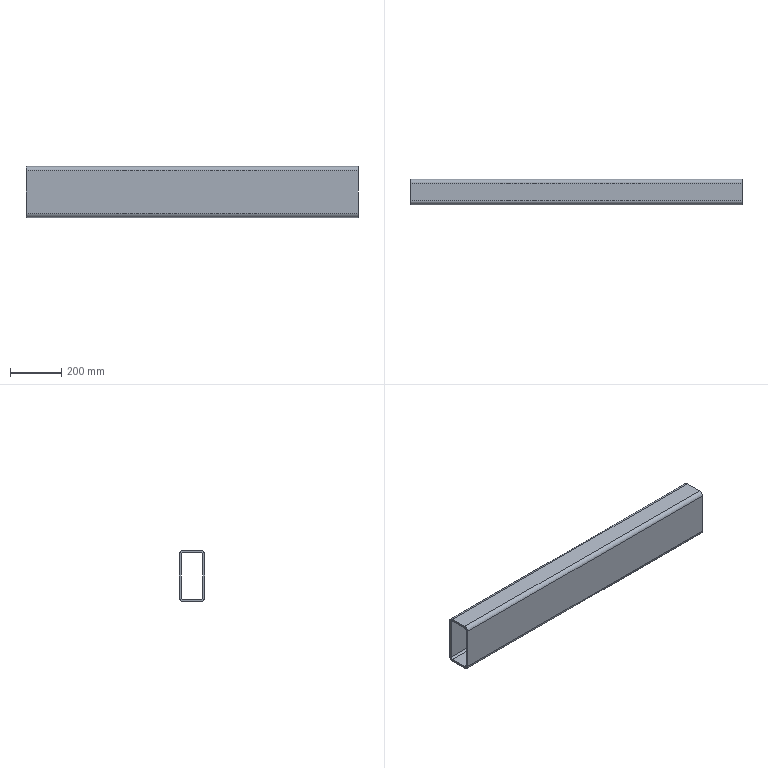Part | STEP file | 01-Column (flat tube 200x100x8)_default<machining> | 1 solid | 18 faces | box 1300 x 100 x 200 mm | volume 5692942 mm3 | plane 10 | cylinder 8 | commonest cylinder face diameters 16 x4 32 x4
STEP:
#1=CARTESIAN_POINT('',(0.,0.,0.));
#2=DIRECTION('',(0.,0.,1.));
#3=DIRECTION('',(1.,0.,0.));
#4=AXIS2_PLACEMENT_3D('',#1,#2,#3);
#5=CARTESIAN_POINT('',(0.,50.,84.));
#6=VERTEX_POINT('',#5);
#7=CARTESIAN_POINT('',(0.,34.,100.));
#8=VERTEX_POINT('',#7);
#9=CARTESIAN_POINT('',(0.,34.,84.));
#10=DIRECTION('',(1.,0.,0.));
#11=DIRECTION('',(0.,0.,-1.));
#12=AXIS2_PLACEMENT_3D('',#9,#10,#11);
#13=CIRCLE('',#12,16.);
#14=CARTESIAN_POINT('',(1300.,34.,84.));
#15=DIRECTION('',(-1.,0.,0.));
#16=DIRECTION('',(0.,0.,1.));
#17=AXIS2_PLACEMENT_3D('',#14,#15,#16);
#18=CYLINDRICAL_SURFACE('',#17,16.);
#19=CARTESIAN_POINT('',(3.142,1300.));
#20=DIRECTION('',(-1.,0.));
#21=VECTOR('',#20,1.);
#22=LINE('',#19,#21);
#23=(GEOMETRIC_REPRESENTATION_CONTEXT(2)PARAMETRIC_REPRESENTATION_CONTEXT()REPRESENTATION_CONTEXT('',''));
#24=DEFINITIONAL_REPRESENTATION('',(#22),#23);
#25=PCURVE('',#18,#24);
#26=CARTESIAN_POINT('',(0.,34.,84.));
#27=DIRECTION('',(1.,0.,0.));
#28=DIRECTION('',(0.,0.,-1.));
#29=AXIS2_PLACEMENT_3D('',#26,#27,#28);
#30=PLANE('',#29);
#31=CARTESIAN_POINT('',(0.,0.));
#32=DIRECTION('',(1.,0.));
#33=AXIS2_PLACEMENT_2D('',#31,#32);
#34=CIRCLE('',#33,16.);
#35=(GEOMETRIC_REPRESENTATION_CONTEXT(2)PARAMETRIC_REPRESENTATION_CONTEXT()REPRESENTATION_CONTEXT('',''));
#36=DEFINITIONAL_REPRESENTATION('',(#34),#35);
#37=PCURVE('',#30,#36);
#38=SURFACE_CURVE('',#13,(#25,#37),.PCURVE_S1.);
#39=EDGE_CURVE('',#6,#8,#38,.T.);
#40=ORIENTED_EDGE('',*,*,#39,.T.);
#41=CARTESIAN_POINT('',(1300.,34.,100.));
#42=VERTEX_POINT('',#41);
#43=CARTESIAN_POINT('',(1300.,34.,100.));
#44=DIRECTION('',(-1.,0.,0.));
#45=VECTOR('',#44,1.);
#46=LINE('',#43,#45);
#47=CARTESIAN_POINT('',(0.,0.));
#48=DIRECTION('',(0.,1.));
#49=VECTOR('',#48,1.);
#50=LINE('',#47,#49);
#51=(GEOMETRIC_REPRESENTATION_CONTEXT(2)PARAMETRIC_REPRESENTATION_CONTEXT()REPRESENTATION_CONTEXT('',''));
#52=DEFINITIONAL_REPRESENTATION('',(#50),#51);
#53=PCURVE('',#18,#52);
#54=CARTESIAN_POINT('',(1300.,34.,100.));
#55=DIRECTION('',(0.,0.,-1.));
#56=DIRECTION('',(-1.,0.,0.));
#57=AXIS2_PLACEMENT_3D('',#54,#55,#56);
#58=PLANE('',#57);
#59=CARTESIAN_POINT('',(0.,0.));
#60=DIRECTION('',(1.,0.));
#61=VECTOR('',#60,1.);
#62=LINE('',#59,#61);
#63=(GEOMETRIC_REPRESENTATION_CONTEXT(2)PARAMETRIC_REPRESENTATION_CONTEXT()REPRESENTATION_CONTEXT('',''));
#64=DEFINITIONAL_REPRESENTATION('',(#62),#63);
#65=PCURVE('',#58,#64);
#66=SURFACE_CURVE('',#46,(#53,#65),.PCURVE_S1.);
#67=EDGE_CURVE('',#42,#8,#66,.T.);
#68=ORIENTED_EDGE('',*,*,#67,.F.);
#69=CARTESIAN_POINT('',(1300.,50.,84.));
#70=VERTEX_POINT('',#69);
#71=CARTESIAN_POINT('',(1300.,34.,84.));
#72=DIRECTION('',(1.,0.,0.));
#73=DIRECTION('',(0.,0.,-1.));
#74=AXIS2_PLACEMENT_3D('',#71,#72,#73);
#75=CIRCLE('',#74,16.);
#76=CARTESIAN_POINT('',(3.142,0.));
#77=DIRECTION('',(-1.,0.));
#78=VECTOR('',#77,1.);
#79=LINE('',#76,#78);
#80=(GEOMETRIC_REPRESENTATION_CONTEXT(2)PARAMETRIC_REPRESENTATION_CONTEXT()REPRESENTATION_CONTEXT('',''));
#81=DEFINITIONAL_REPRESENTATION('',(#79),#80);
#82=PCURVE('',#18,#81);
#83=CARTESIAN_POINT('',(1300.,34.,84.));
#84=DIRECTION('',(1.,0.,0.));
#85=DIRECTION('',(0.,0.,-1.));
#86=AXIS2_PLACEMENT_3D('',#83,#84,#85);
#87=PLANE('',#86);
#88=CARTESIAN_POINT('',(0.,0.));
#89=DIRECTION('',(1.,0.));
#90=AXIS2_PLACEMENT_2D('',#88,#89);
#91=CIRCLE('',#90,16.);
#92=(GEOMETRIC_REPRESENTATION_CONTEXT(2)PARAMETRIC_REPRESENTATION_CONTEXT()REPRESENTATION_CONTEXT('',''));
#93=DEFINITIONAL_REPRESENTATION('',(#91),#92);
#94=PCURVE('',#87,#93);
#95=SURFACE_CURVE('',#75,(#82,#94),.PCURVE_S1.);
#96=EDGE_CURVE('',#70,#42,#95,.T.);
#97=ORIENTED_EDGE('',*,*,#96,.F.);
#98=CARTESIAN_POINT('',(1300.,50.,84.));
#99=DIRECTION('',(-1.,0.,0.));
#100=VECTOR('',#99,1.);
#101=LINE('',#98,#100);
#102=CARTESIAN_POINT('',(1.571,0.));
#103=DIRECTION('',(0.,1.));
#104=VECTOR('',#103,1.);
#105=LINE('',#102,#104);
#106=(GEOMETRIC_REPRESENTATION_CONTEXT(2)PARAMETRIC_REPRESENTATION_CONTEXT()REPRESENTATION_CONTEXT('',''));
#107=DEFINITIONAL_REPRESENTATION('',(#105),#106);
#108=PCURVE('',#18,#107);
#109=CARTESIAN_POINT('',(1300.,50.,84.));
#110=DIRECTION('',(0.,-1.,0.));
#111=DIRECTION('',(0.,0.,-1.));
#112=AXIS2_PLACEMENT_3D('',#109,#110,#111);
#113=PLANE('',#112);
#114=CARTESIAN_POINT('',(0.,0.));
#115=DIRECTION('',(0.,-1.));
#116=VECTOR('',#115,1.);
#117=LINE('',#114,#116);
#118=(GEOMETRIC_REPRESENTATION_CONTEXT(2)PARAMETRIC_REPRESENTATION_CONTEXT()REPRESENTATION_CONTEXT('',''));
#119=DEFINITIONAL_REPRESENTATION('',(#117),#118);
#120=PCURVE('',#113,#119);
#121=SURFACE_CURVE('',#101,(#108,#120),.PCURVE_S1.);
#122=EDGE_CURVE('',#70,#6,#121,.T.);
#123=ORIENTED_EDGE('',*,*,#122,.T.);
#124=EDGE_LOOP('',(#40,#68,#97,#123));
#125=FACE_BOUND('',#124,.T.);
#126=ADVANCED_FACE('',(#125),#18,.T.);
#127=CARTESIAN_POINT('',(0.,-34.,100.));
#128=VERTEX_POINT('',#127);
#129=CARTESIAN_POINT('',(0.,34.,100.));
#130=DIRECTION('',(0.,-1.,0.));
#131=VECTOR('',#130,1.);
#132=LINE('',#129,#131);
#133=CARTESIAN_POINT('',(1300.,0.));
#134=DIRECTION('',(0.,-1.));
#135=VECTOR('',#134,1.);
#136=LINE('',#133,#135);
#137=(GEOMETRIC_REPRESENTATION_CONTEXT(2)PARAMETRIC_REPRESENTATION_CONTEXT()REPRESENTATION_CONTEXT('',''));
#138=DEFINITIONAL_REPRESENTATION('',(#136),#137);
#139=PCURVE('',#58,#138);
#140=CARTESIAN_POINT('',(-16.,0.));
#141=DIRECTION('',(0.,-1.));
#142=VECTOR('',#141,1.);
#143=LINE('',#140,#142);
#144=(GEOMETRIC_REPRESENTATION_CONTEXT(2)PARAMETRIC_REPRESENTATION_CONTEXT()REPRESENTATION_CONTEXT('',''));
#145=DEFINITIONAL_REPRESENTATION('',(#143),#144);
#146=PCURVE('',#30,#145);
#147=SURFACE_CURVE('',#132,(#139,#146),.PCURVE_S1.);
#148=EDGE_CURVE('',#8,#128,#147,.T.);
#149=ORIENTED_EDGE('',*,*,#148,.T.);
#150=CARTESIAN_POINT('',(1300.,-34.,100.));
#151=VERTEX_POINT('',#150);
#152=CARTESIAN_POINT('',(1300.,-34.,100.));
#153=DIRECTION('',(-1.,0.,0.));
#154=VECTOR('',#153,1.);
#155=LINE('',#152,#154);
#156=CARTESIAN_POINT('',(0.,-68.));
#157=DIRECTION('',(1.,0.));
#158=VECTOR('',#157,1.);
#159=LINE('',#156,#158);
#160=(GEOMETRIC_REPRESENTATION_CONTEXT(2)PARAMETRIC_REPRESENTATION_CONTEXT()REPRESENTATION_CONTEXT('',''));
#161=DEFINITIONAL_REPRESENTATION('',(#159),#160);
#162=PCURVE('',#58,#161);
#163=CARTESIAN_POINT('',(1300.,-34.,84.));
#164=DIRECTION('',(-1.,0.,0.));
#165=DIRECTION('',(0.,0.,1.));
#166=AXIS2_PLACEMENT_3D('',#163,#164,#165);
#167=CYLINDRICAL_SURFACE('',#166,16.);
#168=CARTESIAN_POINT('',(6.283,0.));
#169=DIRECTION('',(0.,1.));
#170=VECTOR('',#169,1.);
#171=LINE('',#168,#170);
#172=(GEOMETRIC_REPRESENTATION_CONTEXT(2)PARAMETRIC_REPRESENTATION_CONTEXT()REPRESENTATION_CONTEXT('',''));
#173=DEFINITIONAL_REPRESENTATION('',(#171),#172);
#174=PCURVE('',#167,#173);
#175=SURFACE_CURVE('',#155,(#162,#174),.PCURVE_S1.);
#176=EDGE_CURVE('',#151,#128,#175,.T.);
#177=ORIENTED_EDGE('',*,*,#176,.F.);
#178=CARTESIAN_POINT('',(1300.,34.,100.));
#179=DIRECTION('',(0.,-1.,0.));
#180=VECTOR('',#179,1.);
#181=LINE('',#178,#180);
#182=CARTESIAN_POINT('',(0.,0.));
#183=DIRECTION('',(0.,-1.));
#184=VECTOR('',#183,1.);
#185=LINE('',#182,#184);
#186=(GEOMETRIC_REPRESENTATION_CONTEXT(2)PARAMETRIC_REPRESENTATION_CONTEXT()REPRESENTATION_CONTEXT('',''));
#187=DEFINITIONAL_REPRESENTATION('',(#185),#186);
#188=PCURVE('',#58,#187);
#189=CARTESIAN_POINT('',(-16.,0.));
#190=DIRECTION('',(0.,-1.));
#191=VECTOR('',#190,1.);
#192=LINE('',#189,#191);
#193=(GEOMETRIC_REPRESENTATION_CONTEXT(2)PARAMETRIC_REPRESENTATION_CONTEXT()REPRESENTATION_CONTEXT('',''));
#194=DEFINITIONAL_REPRESENTATION('',(#192),#193);
#195=PCURVE('',#87,#194);
#196=SURFACE_CURVE('',#181,(#188,#195),.PCURVE_S1.);
#197=EDGE_CURVE('',#42,#151,#196,.T.);
#198=ORIENTED_EDGE('',*,*,#197,.F.);
#199=ORIENTED_EDGE('',*,*,#67,.T.);
#200=EDGE_LOOP('',(#149,#177,#198,#199));
#201=FACE_BOUND('',#200,.T.);
#202=ADVANCED_FACE('',(#201),#58,.F.);
#203=CARTESIAN_POINT('',(0.,-50.,84.));
#204=VERTEX_POINT('',#203);
#205=CARTESIAN_POINT('',(0.,-34.,84.));
#206=DIRECTION('',(1.,0.,0.));
#207=DIRECTION('',(0.,0.,-1.));
#208=AXIS2_PLACEMENT_3D('',#205,#206,#207);
#209=CIRCLE('',#208,16.);
#210=CARTESIAN_POINT('',(9.425,1300.));
#211=DIRECTION('',(-1.,0.));
#212=VECTOR('',#211,1.);
#213=LINE('',#210,#212);
#214=(GEOMETRIC_REPRESENTATION_CONTEXT(2)PARAMETRIC_REPRESENTATION_CONTEXT()REPRESENTATION_CONTEXT('',''));
#215=DEFINITIONAL_REPRESENTATION('',(#213),#214);
#216=PCURVE('',#167,#215);
#217=CARTESIAN_POINT('',(0.,-68.));
#218=DIRECTION('',(1.,0.));
#219=AXIS2_PLACEMENT_2D('',#217,#218);
#220=CIRCLE('',#219,16.);
#221=(GEOMETRIC_REPRESENTATION_CONTEXT(2)PARAMETRIC_REPRESENTATION_CONTEXT()REPRESENTATION_CONTEXT('',''));
#222=DEFINITIONAL_REPRESENTATION('',(#220),#221);
#223=PCURVE('',#30,#222);
#224=SURFACE_CURVE('',#209,(#216,#223),.PCURVE_S1.);
#225=EDGE_CURVE('',#128,#204,#224,.T.);
#226=ORIENTED_EDGE('',*,*,#225,.T.);
#227=CARTESIAN_POINT('',(1300.,-50.,84.));
#228=VERTEX_POINT('',#227);
#229=CARTESIAN_POINT('',(1300.,-50.,84.));
#230=DIRECTION('',(-1.,0.,0.));
#231=VECTOR('',#230,1.);
#232=LINE('',#229,#231);
#233=CARTESIAN_POINT('',(4.712,0.));
#234=DIRECTION('',(0.,1.));
#235=VECTOR('',#234,1.);
#236=LINE('',#233,#235);
#237=(GEOMETRIC_REPRESENTATION_CONTEXT(2)PARAMETRIC_REPRESENTATION_CONTEXT()REPRESENTATION_CONTEXT('',''));
#238=DEFINITIONAL_REPRESENTATION('',(#236),#237);
#239=PCURVE('',#167,#238);
#240=CARTESIAN_POINT('',(1300.,-50.,-84.));
#241=DIRECTION('',(0.,1.,0.));
#242=DIRECTION('',(0.,0.,1.));
#243=AXIS2_PLACEMENT_3D('',#240,#241,#242);
#244=PLANE('',#243);
#245=CARTESIAN_POINT('',(168.,0.));
#246=DIRECTION('',(0.,-1.));
#247=VECTOR('',#246,1.);
#248=LINE('',#245,#247);
#249=(GEOMETRIC_REPRESENTATION_CONTEXT(2)PARAMETRIC_REPRESENTATION_CONTEXT()REPRESENTATION_CONTEXT('',''));
#250=DEFINITIONAL_REPRESENTATION('',(#248),#249);
#251=PCURVE('',#244,#250);
#252=SURFACE_CURVE('',#232,(#239,#251),.PCURVE_S1.);
#253=EDGE_CURVE('',#228,#204,#252,.T.);
#254=ORIENTED_EDGE('',*,*,#253,.F.);
#255=CARTESIAN_POINT('',(1300.,-34.,84.));
#256=DIRECTION('',(1.,0.,0.));
#257=DIRECTION('',(0.,0.,-1.));
#258=AXIS2_PLACEMENT_3D('',#255,#256,#257);
#259=CIRCLE('',#258,16.);
#260=CARTESIAN_POINT('',(9.425,0.));
#261=DIRECTION('',(-1.,0.));
#262=VECTOR('',#261,1.);
#263=LINE('',#260,#262);
#264=(GEOMETRIC_REPRESENTATION_CONTEXT(2)PARAMETRIC_REPRESENTATION_CONTEXT()REPRESENTATION_CONTEXT('',''));
#265=DEFINITIONAL_REPRESENTATION('',(#263),#264);
#266=PCURVE('',#167,#265);
#267=CARTESIAN_POINT('',(0.,-68.));
#268=DIRECTION('',(1.,0.));
#269=AXIS2_PLACEMENT_2D('',#267,#268);
#270=CIRCLE('',#269,16.);
#271=(GEOMETRIC_REPRESENTATION_CONTEXT(2)PARAMETRIC_REPRESENTATION_CONTEXT()REPRESENTATION_CONTEXT('',''));
#272=DEFINITIONAL_REPRESENTATION('',(#270),#271);
#273=PCURVE('',#87,#272);
#274=SURFACE_CURVE('',#259,(#266,#273),.PCURVE_S1.);
#275=EDGE_CURVE('',#151,#228,#274,.T.);
#276=ORIENTED_EDGE('',*,*,#275,.F.);
#277=ORIENTED_EDGE('',*,*,#176,.T.);
#278=EDGE_LOOP('',(#226,#254,#276,#277));
#279=FACE_BOUND('',#278,.T.);
#280=ADVANCED_FACE('',(#279),#167,.T.);
#281=CARTESIAN_POINT('',(0.,-50.,-84.));
#282=VERTEX_POINT('',#281);
#283=CARTESIAN_POINT('',(0.,-50.,-84.));
#284=DIRECTION('',(0.,0.,-1.));
#285=VECTOR('',#284,1.);
#286=LINE('',#283,#285);
#287=CARTESIAN_POINT('',(0.,-1300.));
#288=DIRECTION('',(-1.,0.));
#289=VECTOR('',#288,1.);
#290=LINE('',#287,#289);
#291=(GEOMETRIC_REPRESENTATION_CONTEXT(2)PARAMETRIC_REPRESENTATION_CONTEXT()REPRESENTATION_CONTEXT('',''));
#292=DEFINITIONAL_REPRESENTATION('',(#290),#291);
#293=PCURVE('',#244,#292);
#294=CARTESIAN_POINT('',(168.,-84.));
#295=DIRECTION('',(1.,0.));
#296=VECTOR('',#295,1.);
#297=LINE('',#294,#296);
#298=(GEOMETRIC_REPRESENTATION_CONTEXT(2)PARAMETRIC_REPRESENTATION_CONTEXT()REPRESENTATION_CONTEXT('',''));
#299=DEFINITIONAL_REPRESENTATION('',(#297),#298);
#300=PCURVE('',#30,#299);
#301=SURFACE_CURVE('',#286,(#293,#300),.PCURVE_S1.);
#302=EDGE_CURVE('',#204,#282,#301,.T.);
#303=ORIENTED_EDGE('',*,*,#302,.T.);
#304=CARTESIAN_POINT('',(1300.,-50.,-84.));
#305=VERTEX_POINT('',#304);
#306=CARTESIAN_POINT('',(1300.,-50.,-84.));
#307=DIRECTION('',(-1.,0.,0.));
#308=VECTOR('',#307,1.);
#309=LINE('',#306,#308);
#310=CARTESIAN_POINT('',(0.,0.));
#311=DIRECTION('',(0.,-1.));
#312=VECTOR('',#311,1.);
#313=LINE('',#310,#312);
#314=(GEOMETRIC_REPRESENTATION_CONTEXT(2)PARAMETRIC_REPRESENTATION_CONTEXT()REPRESENTATION_CONTEXT('',''));
#315=DEFINITIONAL_REPRESENTATION('',(#313),#314);
#316=PCURVE('',#244,#315);
#317=CARTESIAN_POINT('',(1300.,-34.,-84.));
#318=DIRECTION('',(-1.,0.,0.));
#319=DIRECTION('',(0.,0.,1.));
#320=AXIS2_PLACEMENT_3D('',#317,#318,#319);
#321=CYLINDRICAL_SURFACE('',#320,16.);
#322=CARTESIAN_POINT('',(4.712,0.));
#323=DIRECTION('',(0.,1.));
#324=VECTOR('',#323,1.);
#325=LINE('',#322,#324);
#326=(GEOMETRIC_REPRESENTATION_CONTEXT(2)PARAMETRIC_REPRESENTATION_CONTEXT()REPRESENTATION_CONTEXT('',''));
#327=DEFINITIONAL_REPRESENTATION('',(#325),#326);
#328=PCURVE('',#321,#327);
#329=SURFACE_CURVE('',#309,(#316,#328),.PCURVE_S1.);
#330=EDGE_CURVE('',#305,#282,#329,.T.);
#331=ORIENTED_EDGE('',*,*,#330,.F.);
#332=CARTESIAN_POINT('',(1300.,-50.,-84.));
#333=DIRECTION('',(0.,0.,-1.));
#334=VECTOR('',#333,1.);
#335=LINE('',#332,#334);
#336=CARTESIAN_POINT('',(0.,0.));
#337=DIRECTION('',(-1.,0.));
#338=VECTOR('',#337,1.);
#339=LINE('',#336,#338);
#340=(GEOMETRIC_REPRESENTATION_CONTEXT(2)PARAMETRIC_REPRESENTATION_CONTEXT()REPRESENTATION_CONTEXT('',''));
#341=DEFINITIONAL_REPRESENTATION('',(#339),#340);
#342=PCURVE('',#244,#341);
#343=CARTESIAN_POINT('',(168.,-84.));
#344=DIRECTION('',(1.,0.));
#345=VECTOR('',#344,1.);
#346=LINE('',#343,#345);
#347=(GEOMETRIC_REPRESENTATION_CONTEXT(2)PARAMETRIC_REPRESENTATION_CONTEXT()REPRESENTATION_CONTEXT('',''));
#348=DEFINITIONAL_REPRESENTATION('',(#346),#347);
#349=PCURVE('',#87,#348);
#350=SURFACE_CURVE('',#335,(#342,#349),.PCURVE_S1.);
#351=EDGE_CURVE('',#228,#305,#350,.T.);
#352=ORIENTED_EDGE('',*,*,#351,.F.);
#353=ORIENTED_EDGE('',*,*,#253,.T.);
#354=EDGE_LOOP('',(#303,#331,#352,#353));
#355=FACE_BOUND('',#354,.T.);
#356=ADVANCED_FACE('',(#355),#244,.F.);
#357=CARTESIAN_POINT('',(0.,-34.,-100.));
#358=VERTEX_POINT('',#357);
#359=CARTESIAN_POINT('',(0.,-34.,-84.));
#360=DIRECTION('',(1.,0.,0.));
#361=DIRECTION('',(0.,0.,-1.));
#362=AXIS2_PLACEMENT_3D('',#359,#360,#361);
#363=CIRCLE('',#362,16.);
#364=CARTESIAN_POINT('',(9.425,1300.));
#365=DIRECTION('',(-1.,0.));
#366=VECTOR('',#365,1.);
#367=LINE('',#364,#366);
#368=(GEOMETRIC_REPRESENTATION_CONTEXT(2)PARAMETRIC_REPRESENTATION_CONTEXT()REPRESENTATION_CONTEXT('',''));
#369=DEFINITIONAL_REPRESENTATION('',(#367),#368);
#370=PCURVE('',#321,#369);
#371=CARTESIAN_POINT('',(168.,-68.));
#372=DIRECTION('',(1.,0.));
#373=AXIS2_PLACEMENT_2D('',#371,#372);
#374=CIRCLE('',#373,16.);
#375=(GEOMETRIC_REPRESENTATION_CONTEXT(2)PARAMETRIC_REPRESENTATION_CONTEXT()REPRESENTATION_CONTEXT('',''));
#376=DEFINITIONAL_REPRESENTATION('',(#374),#375);
#377=PCURVE('',#30,#376);
#378=SURFACE_CURVE('',#363,(#370,#377),.PCURVE_S1.);
#379=EDGE_CURVE('',#282,#358,#378,.T.);
#380=ORIENTED_EDGE('',*,*,#379,.T.);
#381=CARTESIAN_POINT('',(1300.,-34.,-100.));
#382=VERTEX_POINT('',#381);
#383=CARTESIAN_POINT('',(1300.,-34.,-100.));
#384=DIRECTION('',(-1.,0.,0.));
#385=VECTOR('',#384,1.);
#386=LINE('',#383,#385);
#387=CARTESIAN_POINT('',(3.142,0.));
#388=DIRECTION('',(0.,1.));
#389=VECTOR('',#388,1.);
#390=LINE('',#387,#389);
#391=(GEOMETRIC_REPRESENTATION_CONTEXT(2)PARAMETRIC_REPRESENTATION_CONTEXT()REPRESENTATION_CONTEXT('',''));
#392=DEFINITIONAL_REPRESENTATION('',(#390),#391);
#393=PCURVE('',#321,#392);
#394=CARTESIAN_POINT('',(1300.,-34.,-100.));
#395=DIRECTION('',(0.,0.,1.));
#396=DIRECTION('',(1.,0.,0.));
#397=AXIS2_PLACEMENT_3D('',#394,#395,#396);
#398=PLANE('',#397);
#399=CARTESIAN_POINT('',(0.,0.));
#400=DIRECTION('',(-1.,0.));
#401=VECTOR('',#400,1.);
#402=LINE('',#399,#401);
#403=(GEOMETRIC_REPRESENTATION_CONTEXT(2)PARAMETRIC_REPRESENTATION_CONTEXT()REPRESENTATION_CONTEXT('',''));
#404=DEFINITIONAL_REPRESENTATION('',(#402),#403);
#405=PCURVE('',#398,#404);
#406=SURFACE_CURVE('',#386,(#393,#405),.PCURVE_S1.);
#407=EDGE_CURVE('',#382,#358,#406,.T.);
#408=ORIENTED_EDGE('',*,*,#407,.F.);
#409=CARTESIAN_POINT('',(1300.,-34.,-84.));
#410=DIRECTION('',(1.,0.,0.));
#411=DIRECTION('',(0.,0.,-1.));
#412=AXIS2_PLACEMENT_3D('',#409,#410,#411);
#413=CIRCLE('',#412,16.);
#414=CARTESIAN_POINT('',(9.425,0.));
#415=DIRECTION('',(-1.,0.));
#416=VECTOR('',#415,1.);
#417=LINE('',#414,#416);
#418=(GEOMETRIC_REPRESENTATION_CONTEXT(2)PARAMETRIC_REPRESENTATION_CONTEXT()REPRESENTATION_CONTEXT('',''));
#419=DEFINITIONAL_REPRESENTATION('',(#417),#418);
#420=PCURVE('',#321,#419);
#421=CARTESIAN_POINT('',(168.,-68.));
#422=DIRECTION('',(1.,0.));
#423=AXIS2_PLACEMENT_2D('',#421,#422);
#424=CIRCLE('',#423,16.);
#425=(GEOMETRIC_REPRESENTATION_CONTEXT(2)PARAMETRIC_REPRESENTATION_CONTEXT()REPRESENTATION_CONTEXT('',''));
#426=DEFINITIONAL_REPRESENTATION('',(#424),#425);
#427=PCURVE('',#87,#426);
#428=SURFACE_CURVE('',#413,(#420,#427),.PCURVE_S1.);
#429=EDGE_CURVE('',#305,#382,#428,.T.);
#430=ORIENTED_EDGE('',*,*,#429,.F.);
#431=ORIENTED_EDGE('',*,*,#330,.T.);
#432=EDGE_LOOP('',(#380,#408,#430,#431));
#433=FACE_BOUND('',#432,.T.);
#434=ADVANCED_FACE('',(#433),#321,.T.);
#435=CARTESIAN_POINT('',(0.,34.,-100.));
#436=VERTEX_POINT('',#435);
#437=CARTESIAN_POINT('',(0.,-34.,-100.));
#438=DIRECTION('',(0.,1.,0.));
#439=VECTOR('',#438,1.);
#440=LINE('',#437,#439);
#441=CARTESIAN_POINT('',(-1300.,0.));
#442=DIRECTION('',(0.,1.));
#443=VECTOR('',#442,1.);
#444=LINE('',#441,#443);
#445=(GEOMETRIC_REPRESENTATION_CONTEXT(2)PARAMETRIC_REPRESENTATION_CONTEXT()REPRESENTATION_CONTEXT('',''));
#446=DEFINITIONAL_REPRESENTATION('',(#444),#445);
#447=PCURVE('',#398,#446);
#448=CARTESIAN_POINT('',(184.,-68.));
#449=DIRECTION('',(0.,1.));
#450=VECTOR('',#449,1.);
#451=LINE('',#448,#450);
#452=(GEOMETRIC_REPRESENTATION_CONTEXT(2)PARAMETRIC_REPRESENTATION_CONTEXT()REPRESENTATION_CONTEXT('',''));
#453=DEFINITIONAL_REPRESENTATION('',(#451),#452);
#454=PCURVE('',#30,#453);
#455=SURFACE_CURVE('',#440,(#447,#454),.PCURVE_S1.);
#456=EDGE_CURVE('',#358,#436,#455,.T.);
#457=ORIENTED_EDGE('',*,*,#456,.T.);
#458=CARTESIAN_POINT('',(1300.,34.,-100.));
#459=VERTEX_POINT('',#458);
#460=CARTESIAN_POINT('',(1300.,34.,-100.));
#461=DIRECTION('',(-1.,0.,0.));
#462=VECTOR('',#461,1.);
#463=LINE('',#460,#462);
#464=CARTESIAN_POINT('',(0.,68.));
#465=DIRECTION('',(-1.,0.));
#466=VECTOR('',#465,1.);
#467=LINE('',#464,#466);
#468=(GEOMETRIC_REPRESENTATION_CONTEXT(2)PARAMETRIC_REPRESENTATION_CONTEXT()REPRESENTATION_CONTEXT('',''));
#469=DEFINITIONAL_REPRESENTATION('',(#467),#468);
#470=PCURVE('',#398,#469);
#471=CARTESIAN_POINT('',(1300.,34.,-84.));
#472=DIRECTION('',(-1.,0.,0.));
#473=DIRECTION('',(0.,0.,1.));
#474=AXIS2_PLACEMENT_3D('',#471,#472,#473);
#475=CYLINDRICAL_SURFACE('',#474,16.);
#476=CARTESIAN_POINT('',(3.142,0.));
#477=DIRECTION('',(0.,1.));
#478=VECTOR('',#477,1.);
#479=LINE('',#476,#478);
#480=(GEOMETRIC_REPRESENTATION_CONTEXT(2)PARAMETRIC_REPRESENTATION_CONTEXT()REPRESENTATION_CONTEXT('',''));
#481=DEFINITIONAL_REPRESENTATION('',(#479),#480);
#482=PCURVE('',#475,#481);
#483=SURFACE_CURVE('',#463,(#470,#482),.PCURVE_S1.);
#484=EDGE_CURVE('',#459,#436,#483,.T.);
#485=ORIENTED_EDGE('',*,*,#484,.F.);
#486=CARTESIAN_POINT('',(1300.,-34.,-100.));
#487=DIRECTION('',(0.,1.,0.));
#488=VECTOR('',#487,1.);
#489=LINE('',#486,#488);
#490=CARTESIAN_POINT('',(0.,0.));
#491=DIRECTION('',(0.,1.));
#492=VECTOR('',#491,1.);
#493=LINE('',#490,#492);
#494=(GEOMETRIC_REPRESENTATION_CONTEXT(2)PARAMETRIC_REPRESENTATION_CONTEXT()REPRESENTATION_CONTEXT('',''));
#495=DEFINITIONAL_REPRESENTATION('',(#493),#494);
#496=PCURVE('',#398,#495);
#497=CARTESIAN_POINT('',(184.,-68.));
#498=DIRECTION('',(0.,1.));
#499=VECTOR('',#498,1.);
#500=LINE('',#497,#499);
#501=(GEOMETRIC_REPRESENTATION_CONTEXT(2)PARAMETRIC_REPRESENTATION_CONTEXT()REPRESENTATION_CONTEXT('',''));
#502=DEFINITIONAL_REPRESENTATION('',(#500),#501);
#503=PCURVE('',#87,#502);
#504=SURFACE_CURVE('',#489,(#496,#503),.PCURVE_S1.);
#505=EDGE_CURVE('',#382,#459,#504,.T.);
#506=ORIENTED_EDGE('',*,*,#505,.F.);
#507=ORIENTED_EDGE('',*,*,#407,.T.);
#508=EDGE_LOOP('',(#457,#485,#506,#507));
#509=FACE_BOUND('',#508,.T.);
#510=ADVANCED_FACE('',(#509),#398,.F.);
#511=CARTESIAN_POINT('',(0.,50.,-84.));
#512=VERTEX_POINT('',#511);
#513=CARTESIAN_POINT('',(0.,34.,-84.));
#514=DIRECTION('',(1.,0.,0.));
#515=DIRECTION('',(0.,0.,-1.));
#516=AXIS2_PLACEMENT_3D('',#513,#514,#515);
#517=CIRCLE('',#516,16.);
#518=CARTESIAN_POINT('',(3.142,1300.));
#519=DIRECTION('',(-1.,0.));
#520=VECTOR('',#519,1.);
#521=LINE('',#518,#520);
#522=(GEOMETRIC_REPRESENTATION_CONTEXT(2)PARAMETRIC_REPRESENTATION_CONTEXT()REPRESENTATION_CONTEXT('',''));
#523=DEFINITIONAL_REPRESENTATION('',(#521),#522);
#524=PCURVE('',#475,#523);
#525=CARTESIAN_POINT('',(168.,0.));
#526=DIRECTION('',(1.,0.));
#527=AXIS2_PLACEMENT_2D('',#525,#526);
#528=CIRCLE('',#527,16.);
#529=(GEOMETRIC_REPRESENTATION_CONTEXT(2)PARAMETRIC_REPRESENTATION_CONTEXT()REPRESENTATION_CONTEXT('',''));
#530=DEFINITIONAL_REPRESENTATION('',(#528),#529);
#531=PCURVE('',#30,#530);
#532=SURFACE_CURVE('',#517,(#524,#531),.PCURVE_S1.);
#533=EDGE_CURVE('',#436,#512,#532,.T.);
#534=ORIENTED_EDGE('',*,*,#533,.T.);
#535=CARTESIAN_POINT('',(1300.,50.,-84.));
#536=VERTEX_POINT('',#535);
#537=CARTESIAN_POINT('',(1300.,50.,-84.));
#538=DIRECTION('',(-1.,0.,0.));
#539=VECTOR('',#538,1.);
#540=LINE('',#537,#539);
#541=CARTESIAN_POINT('',(1.571,0.));
#542=DIRECTION('',(0.,1.));
#543=VECTOR('',#542,1.);
#544=LINE('',#541,#543);
#545=(GEOMETRIC_REPRESENTATION_CONTEXT(2)PARAMETRIC_REPRESENTATION_CONTEXT()REPRESENTATION_CONTEXT('',''));
#546=DEFINITIONAL_REPRESENTATION('',(#544),#545);
#547=PCURVE('',#475,#546);
#548=CARTESIAN_POINT('',(168.,0.));
#549=DIRECTION('',(0.,-1.));
#550=VECTOR('',#549,1.);
#551=LINE('',#548,#550);
#552=(GEOMETRIC_REPRESENTATION_CONTEXT(2)PARAMETRIC_REPRESENTATION_CONTEXT()REPRESENTATION_CONTEXT('',''));
#553=DEFINITIONAL_REPRESENTATION('',(#551),#552);
#554=PCURVE('',#113,#553);
#555=SURFACE_CURVE('',#540,(#547,#554),.PCURVE_S1.);
#556=EDGE_CURVE('',#536,#512,#555,.T.);
#557=ORIENTED_EDGE('',*,*,#556,.F.);
#558=CARTESIAN_POINT('',(1300.,34.,-84.));
#559=DIRECTION('',(1.,0.,0.));
#560=DIRECTION('',(0.,0.,-1.));
#561=AXIS2_PLACEMENT_3D('',#558,#559,#560);
#562=CIRCLE('',#561,16.);
#563=CARTESIAN_POINT('',(3.142,0.));
#564=DIRECTION('',(-1.,0.));
#565=VECTOR('',#564,1.);
#566=LINE('',#563,#565);
#567=(GEOMETRIC_REPRESENTATION_CONTEXT(2)PARAMETRIC_REPRESENTATION_CONTEXT()REPRESENTATION_CONTEXT('',''));
#568=DEFINITIONAL_REPRESENTATION('',(#566),#567);
#569=PCURVE('',#475,#568);
#570=CARTESIAN_POINT('',(168.,0.));
#571=DIRECTION('',(1.,0.));
#572=AXIS2_PLACEMENT_2D('',#570,#571);
#573=CIRCLE('',#572,16.);
#574=(GEOMETRIC_REPRESENTATION_CONTEXT(2)PARAMETRIC_REPRESENTATION_CONTEXT()REPRESENTATION_CONTEXT('',''));
#575=DEFINITIONAL_REPRESENTATION('',(#573),#574);
#576=PCURVE('',#87,#575);
#577=SURFACE_CURVE('',#562,(#569,#576),.PCURVE_S1.);
#578=EDGE_CURVE('',#459,#536,#577,.T.);
#579=ORIENTED_EDGE('',*,*,#578,.F.);
#580=ORIENTED_EDGE('',*,*,#484,.T.);
#581=EDGE_LOOP('',(#534,#557,#579,#580));
#582=FACE_BOUND('',#581,.T.);
#583=ADVANCED_FACE('',(#582),#475,.T.);
#584=CARTESIAN_POINT('',(1300.,-42.,84.));
#585=VERTEX_POINT('',#584);
#586=CARTESIAN_POINT('',(0.,-42.,84.));
#587=VERTEX_POINT('',#586);
#588=CARTESIAN_POINT('',(1300.,-42.,84.));
#589=DIRECTION('',(-1.,0.,0.));
#590=VECTOR('',#589,1.);
#591=LINE('',#588,#590);
#592=CARTESIAN_POINT('',(1300.,-34.,84.));
#593=DIRECTION('',(-1.,0.,0.));
#594=DIRECTION('',(0.,0.,1.));
#595=AXIS2_PLACEMENT_3D('',#592,#593,#594);
#596=CYLINDRICAL_SURFACE('',#595,8.);
#597=CARTESIAN_POINT('',(4.712,0.));
#598=DIRECTION('',(0.,1.));
#599=VECTOR('',#598,1.);
#600=LINE('',#597,#599);
#601=(GEOMETRIC_REPRESENTATION_CONTEXT(2)PARAMETRIC_REPRESENTATION_CONTEXT()REPRESENTATION_CONTEXT('',''));
#602=DEFINITIONAL_REPRESENTATION('',(#600),#601);
#603=PCURVE('',#596,#602);
#604=CARTESIAN_POINT('',(1300.,-42.,-84.));
#605=DIRECTION('',(0.,1.,0.));
#606=DIRECTION('',(0.,0.,1.));
#607=AXIS2_PLACEMENT_3D('',#604,#605,#606);
#608=PLANE('',#607);
#609=CARTESIAN_POINT('',(168.,0.));
#610=DIRECTION('',(0.,-1.));
#611=VECTOR('',#610,1.);
#612=LINE('',#609,#611);
#613=(GEOMETRIC_REPRESENTATION_CONTEXT(2)PARAMETRIC_REPRESENTATION_CONTEXT()REPRESENTATION_CONTEXT('',''));
#614=DEFINITIONAL_REPRESENTATION('',(#612),#613);
#615=PCURVE('',#608,#614);
#616=SURFACE_CURVE('',#591,(#603,#615),.PCURVE_S1.);
#617=EDGE_CURVE('',#585,#587,#616,.T.);
#618=ORIENTED_EDGE('',*,*,#617,.F.);
#619=CARTESIAN_POINT('',(1300.,-34.,92.));
#620=VERTEX_POINT('',#619);
#621=CARTESIAN_POINT('',(1300.,-34.,84.));
#622=DIRECTION('',(1.,0.,0.));
#623=DIRECTION('',(0.,0.,-1.));
#624=AXIS2_PLACEMENT_3D('',#621,#622,#623);
#625=CIRCLE('',#624,8.);
#626=CARTESIAN_POINT('',(9.425,0.));
#627=DIRECTION('',(-1.,0.));
#628=VECTOR('',#627,1.);
#629=LINE('',#626,#628);
#630=(GEOMETRIC_REPRESENTATION_CONTEXT(2)PARAMETRIC_REPRESENTATION_CONTEXT()REPRESENTATION_CONTEXT('',''));
#631=DEFINITIONAL_REPRESENTATION('',(#629),#630);
#632=PCURVE('',#596,#631);
#633=CARTESIAN_POINT('',(0.,-68.));
#634=DIRECTION('',(1.,0.));
#635=AXIS2_PLACEMENT_2D('',#633,#634);
#636=CIRCLE('',#635,8.);
#637=(GEOMETRIC_REPRESENTATION_CONTEXT(2)PARAMETRIC_REPRESENTATION_CONTEXT()REPRESENTATION_CONTEXT('',''));
#638=DEFINITIONAL_REPRESENTATION('',(#636),#637);
#639=PCURVE('',#87,#638);
#640=SURFACE_CURVE('',#625,(#632,#639),.PCURVE_S1.);
#641=EDGE_CURVE('',#620,#585,#640,.T.);
#642=ORIENTED_EDGE('',*,*,#641,.F.);
#643=CARTESIAN_POINT('',(0.,-34.,92.));
#644=VERTEX_POINT('',#643);
#645=CARTESIAN_POINT('',(1300.,-34.,92.));
#646=DIRECTION('',(-1.,0.,0.));
#647=VECTOR('',#646,1.);
#648=LINE('',#645,#647);
#649=CARTESIAN_POINT('',(6.283,0.));
#650=DIRECTION('',(0.,1.));
#651=VECTOR('',#650,1.);
#652=LINE('',#649,#651);
#653=(GEOMETRIC_REPRESENTATION_CONTEXT(2)PARAMETRIC_REPRESENTATION_CONTEXT()REPRESENTATION_CONTEXT('',''));
#654=DEFINITIONAL_REPRESENTATION('',(#652),#653);
#655=PCURVE('',#596,#654);
#656=CARTESIAN_POINT('',(1300.,34.,92.));
#657=DIRECTION('',(0.,0.,-1.));
#658=DIRECTION('',(-1.,0.,0.));
#659=AXIS2_PLACEMENT_3D('',#656,#657,#658);
#660=PLANE('',#659);
#661=CARTESIAN_POINT('',(0.,-68.));
#662=DIRECTION('',(1.,0.));
#663=VECTOR('',#662,1.);
#664=LINE('',#661,#663);
#665=(GEOMETRIC_REPRESENTATION_CONTEXT(2)PARAMETRIC_REPRESENTATION_CONTEXT()REPRESENTATION_CONTEXT('',''));
#666=DEFINITIONAL_REPRESENTATION('',(#664),#665);
#667=PCURVE('',#660,#666);
#668=SURFACE_CURVE('',#648,(#655,#667),.PCURVE_S1.);
#669=EDGE_CURVE('',#620,#644,#668,.T.);
#670=ORIENTED_EDGE('',*,*,#669,.T.);
#671=CARTESIAN_POINT('',(0.,-34.,84.));
#672=DIRECTION('',(1.,0.,0.));
#673=DIRECTION('',(0.,0.,-1.));
#674=AXIS2_PLACEMENT_3D('',#671,#672,#673);
#675=CIRCLE('',#674,8.);
#676=CARTESIAN_POINT('',(9.425,1300.));
#677=DIRECTION('',(-1.,0.));
#678=VECTOR('',#677,1.);
#679=LINE('',#676,#678);
#680=(GEOMETRIC_REPRESENTATION_CONTEXT(2)PARAMETRIC_REPRESENTATION_CONTEXT()REPRESENTATION_CONTEXT('',''));
#681=DEFINITIONAL_REPRESENTATION('',(#679),#680);
#682=PCURVE('',#596,#681);
#683=CARTESIAN_POINT('',(0.,-68.));
#684=DIRECTION('',(1.,0.));
#685=AXIS2_PLACEMENT_2D('',#683,#684);
#686=CIRCLE('',#685,8.);
#687=(GEOMETRIC_REPRESENTATION_CONTEXT(2)PARAMETRIC_REPRESENTATION_CONTEXT()REPRESENTATION_CONTEXT('',''));
#688=DEFINITIONAL_REPRESENTATION('',(#686),#687);
#689=PCURVE('',#30,#688);
#690=SURFACE_CURVE('',#675,(#682,#689),.PCURVE_S1.);
#691=EDGE_CURVE('',#644,#587,#690,.T.);
#692=ORIENTED_EDGE('',*,*,#691,.T.);
#693=EDGE_LOOP('',(#618,#642,#670,#692));
#694=FACE_BOUND('',#693,.F.);
#695=ADVANCED_FACE('',(#694),#596,.F.);
#696=CARTESIAN_POINT('',(0.,34.,92.));
#697=VERTEX_POINT('',#696);
#698=CARTESIAN_POINT('',(0.,34.,92.));
#699=DIRECTION('',(0.,-1.,0.));
#700=VECTOR('',#699,1.);
#701=LINE('',#698,#700);
#702=CARTESIAN_POINT('',(1300.,0.));
#703=DIRECTION('',(0.,-1.));
#704=VECTOR('',#703,1.);
#705=LINE('',#702,#704);
#706=(GEOMETRIC_REPRESENTATION_CONTEXT(2)PARAMETRIC_REPRESENTATION_CONTEXT()REPRESENTATION_CONTEXT('',''));
#707=DEFINITIONAL_REPRESENTATION('',(#705),#706);
#708=PCURVE('',#660,#707);
#709=CARTESIAN_POINT('',(-8.,0.));
#710=DIRECTION('',(0.,-1.));
#711=VECTOR('',#710,1.);
#712=LINE('',#709,#711);
#713=(GEOMETRIC_REPRESENTATION_CONTEXT(2)PARAMETRIC_REPRESENTATION_CONTEXT()REPRESENTATION_CONTEXT('',''));
#714=DEFINITIONAL_REPRESENTATION('',(#712),#713);
#715=PCURVE('',#30,#714);
#716=SURFACE_CURVE('',#701,(#708,#715),.PCURVE_S1.);
#717=EDGE_CURVE('',#697,#644,#716,.T.);
#718=ORIENTED_EDGE('',*,*,#717,.F.);
#719=CARTESIAN_POINT('',(1300.,34.,92.));
#720=VERTEX_POINT('',#719);
#721=CARTESIAN_POINT('',(1300.,34.,92.));
#722=DIRECTION('',(-1.,0.,0.));
#723=VECTOR('',#722,1.);
#724=LINE('',#721,#723);
#725=CARTESIAN_POINT('',(0.,0.));
#726=DIRECTION('',(1.,0.));
#727=VECTOR('',#726,1.);
#728=LINE('',#725,#727);
#729=(GEOMETRIC_REPRESENTATION_CONTEXT(2)PARAMETRIC_REPRESENTATION_CONTEXT()REPRESENTATION_CONTEXT('',''));
#730=DEFINITIONAL_REPRESENTATION('',(#728),#729);
#731=PCURVE('',#660,#730);
#732=CARTESIAN_POINT('',(1300.,34.,84.));
#733=DIRECTION('',(-1.,0.,0.));
#734=DIRECTION('',(0.,0.,1.));
#735=AXIS2_PLACEMENT_3D('',#732,#733,#734);
#736=CYLINDRICAL_SURFACE('',#735,8.);
#737=CARTESIAN_POINT('',(0.,0.));
#738=DIRECTION('',(0.,1.));
#739=VECTOR('',#738,1.);
#740=LINE('',#737,#739);
#741=(GEOMETRIC_REPRESENTATION_CONTEXT(2)PARAMETRIC_REPRESENTATION_CONTEXT()REPRESENTATION_CONTEXT('',''));
#742=DEFINITIONAL_REPRESENTATION('',(#740),#741);
#743=PCURVE('',#736,#742);
#744=SURFACE_CURVE('',#724,(#731,#743),.PCURVE_S1.);
#745=EDGE_CURVE('',#720,#697,#744,.T.);
#746=ORIENTED_EDGE('',*,*,#745,.F.);
#747=CARTESIAN_POINT('',(1300.,34.,92.));
#748=DIRECTION('',(0.,-1.,0.));
#749=VECTOR('',#748,1.);
#750=LINE('',#747,#749);
#751=CARTESIAN_POINT('',(0.,0.));
#752=DIRECTION('',(0.,-1.));
#753=VECTOR('',#752,1.);
#754=LINE('',#751,#753);
#755=(GEOMETRIC_REPRESENTATION_CONTEXT(2)PARAMETRIC_REPRESENTATION_CONTEXT()REPRESENTATION_CONTEXT('',''));
#756=DEFINITIONAL_REPRESENTATION('',(#754),#755);
#757=PCURVE('',#660,#756);
#758=CARTESIAN_POINT('',(-8.,0.));
#759=DIRECTION('',(0.,-1.));
#760=VECTOR('',#759,1.);
#761=LINE('',#758,#760);
#762=(GEOMETRIC_REPRESENTATION_CONTEXT(2)PARAMETRIC_REPRESENTATION_CONTEXT()REPRESENTATION_CONTEXT('',''));
#763=DEFINITIONAL_REPRESENTATION('',(#761),#762);
#764=PCURVE('',#87,#763);
#765=SURFACE_CURVE('',#750,(#757,#764),.PCURVE_S1.);
#766=EDGE_CURVE('',#720,#620,#765,.T.);
#767=ORIENTED_EDGE('',*,*,#766,.T.);
#768=ORIENTED_EDGE('',*,*,#669,.T.);
#769=EDGE_LOOP('',(#718,#746,#767,#768));
#770=FACE_BOUND('',#769,.T.);
#771=ADVANCED_FACE('',(#770),#660,.T.);
#772=ORIENTED_EDGE('',*,*,#745,.F.);
#773=CARTESIAN_POINT('',(1300.,42.,84.));
#774=VERTEX_POINT('',#773);
#775=CARTESIAN_POINT('',(1300.,34.,84.));
#776=DIRECTION('',(1.,0.,0.));
#777=DIRECTION('',(0.,0.,-1.));
#778=AXIS2_PLACEMENT_3D('',#775,#776,#777);
#779=CIRCLE('',#778,8.);
#780=CARTESIAN_POINT('',(3.142,0.));
#781=DIRECTION('',(-1.,0.));
#782=VECTOR('',#781,1.);
#783=LINE('',#780,#782);
#784=(GEOMETRIC_REPRESENTATION_CONTEXT(2)PARAMETRIC_REPRESENTATION_CONTEXT()REPRESENTATION_CONTEXT('',''));
#785=DEFINITIONAL_REPRESENTATION('',(#783),#784);
#786=PCURVE('',#736,#785);
#787=CARTESIAN_POINT('',(0.,0.));
#788=DIRECTION('',(1.,0.));
#789=AXIS2_PLACEMENT_2D('',#787,#788);
#790=CIRCLE('',#789,8.);
#791=(GEOMETRIC_REPRESENTATION_CONTEXT(2)PARAMETRIC_REPRESENTATION_CONTEXT()REPRESENTATION_CONTEXT('',''));
#792=DEFINITIONAL_REPRESENTATION('',(#790),#791);
#793=PCURVE('',#87,#792);
#794=SURFACE_CURVE('',#779,(#786,#793),.PCURVE_S1.);
#795=EDGE_CURVE('',#774,#720,#794,.T.);
#796=ORIENTED_EDGE('',*,*,#795,.F.);
#797=CARTESIAN_POINT('',(0.,42.,84.));
#798=VERTEX_POINT('',#797);
#799=CARTESIAN_POINT('',(1300.,42.,84.));
#800=DIRECTION('',(-1.,0.,0.));
#801=VECTOR('',#800,1.);
#802=LINE('',#799,#801);
#803=CARTESIAN_POINT('',(1.571,0.));
#804=DIRECTION('',(0.,1.));
#805=VECTOR('',#804,1.);
#806=LINE('',#803,#805);
#807=(GEOMETRIC_REPRESENTATION_CONTEXT(2)PARAMETRIC_REPRESENTATION_CONTEXT()REPRESENTATION_CONTEXT('',''));
#808=DEFINITIONAL_REPRESENTATION('',(#806),#807);
#809=PCURVE('',#736,#808);
#810=CARTESIAN_POINT('',(1300.,42.,84.));
#811=DIRECTION('',(0.,-1.,0.));
#812=DIRECTION('',(0.,0.,-1.));
#813=AXIS2_PLACEMENT_3D('',#810,#811,#812);
#814=PLANE('',#813);
#815=CARTESIAN_POINT('',(0.,0.));
#816=DIRECTION('',(0.,-1.));
#817=VECTOR('',#816,1.);
#818=LINE('',#815,#817);
#819=(GEOMETRIC_REPRESENTATION_CONTEXT(2)PARAMETRIC_REPRESENTATION_CONTEXT()REPRESENTATION_CONTEXT('',''));
#820=DEFINITIONAL_REPRESENTATION('',(#818),#819);
#821=PCURVE('',#814,#820);
#822=SURFACE_CURVE('',#802,(#809,#821),.PCURVE_S1.);
#823=EDGE_CURVE('',#774,#798,#822,.T.);
#824=ORIENTED_EDGE('',*,*,#823,.T.);
#825=CARTESIAN_POINT('',(0.,34.,84.));
#826=DIRECTION('',(1.,0.,0.));
#827=DIRECTION('',(0.,0.,-1.));
#828=AXIS2_PLACEMENT_3D('',#825,#826,#827);
#829=CIRCLE('',#828,8.);
#830=CARTESIAN_POINT('',(3.142,1300.));
#831=DIRECTION('',(-1.,0.));
#832=VECTOR('',#831,1.);
#833=LINE('',#830,#832);
#834=(GEOMETRIC_REPRESENTATION_CONTEXT(2)PARAMETRIC_REPRESENTATION_CONTEXT()REPRESENTATION_CONTEXT('',''));
#835=DEFINITIONAL_REPRESENTATION('',(#833),#834);
#836=PCURVE('',#736,#835);
#837=CARTESIAN_POINT('',(0.,0.));
#838=DIRECTION('',(1.,0.));
#839=AXIS2_PLACEMENT_2D('',#837,#838);
#840=CIRCLE('',#839,8.);
#841=(GEOMETRIC_REPRESENTATION_CONTEXT(2)PARAMETRIC_REPRESENTATION_CONTEXT()REPRESENTATION_CONTEXT('',''));
#842=DEFINITIONAL_REPRESENTATION('',(#840),#841);
#843=PCURVE('',#30,#842);
#844=SURFACE_CURVE('',#829,(#836,#843),.PCURVE_S1.);
#845=EDGE_CURVE('',#798,#697,#844,.T.);
#846=ORIENTED_EDGE('',*,*,#845,.T.);
#847=EDGE_LOOP('',(#772,#796,#824,#846));
#848=FACE_BOUND('',#847,.F.);
#849=ADVANCED_FACE('',(#848),#736,.F.);
#850=CARTESIAN_POINT('',(0.,42.,-84.));
#851=VERTEX_POINT('',#850);
#852=CARTESIAN_POINT('',(0.,42.,84.));
#853=DIRECTION('',(0.,0.,1.));
#854=VECTOR('',#853,1.);
#855=LINE('',#852,#854);
#856=CARTESIAN_POINT('',(0.,-1300.));
#857=DIRECTION('',(-1.,0.));
#858=VECTOR('',#857,1.);
#859=LINE('',#856,#858);
#860=(GEOMETRIC_REPRESENTATION_CONTEXT(2)PARAMETRIC_REPRESENTATION_CONTEXT()REPRESENTATION_CONTEXT('',''));
#861=DEFINITIONAL_REPRESENTATION('',(#859),#860);
#862=PCURVE('',#814,#861);
#863=CARTESIAN_POINT('',(0.,8.));
#864=DIRECTION('',(-1.,0.));
#865=VECTOR('',#864,1.);
#866=LINE('',#863,#865);
#867=(GEOMETRIC_REPRESENTATION_CONTEXT(2)PARAMETRIC_REPRESENTATION_CONTEXT()REPRESENTATION_CONTEXT('',''));
#868=DEFINITIONAL_REPRESENTATION('',(#866),#867);
#869=PCURVE('',#30,#868);
#870=SURFACE_CURVE('',#855,(#862,#869),.PCURVE_S1.);
#871=EDGE_CURVE('',#851,#798,#870,.T.);
#872=ORIENTED_EDGE('',*,*,#871,.F.);
#873=CARTESIAN_POINT('',(1300.,42.,-84.));
#874=VERTEX_POINT('',#873);
#875=CARTESIAN_POINT('',(1300.,42.,-84.));
#876=DIRECTION('',(-1.,0.,0.));
#877=VECTOR('',#876,1.);
#878=LINE('',#875,#877);
#879=CARTESIAN_POINT('',(168.,0.));
#880=DIRECTION('',(0.,-1.));
#881=VECTOR('',#880,1.);
#882=LINE('',#879,#881);
#883=(GEOMETRIC_REPRESENTATION_CONTEXT(2)PARAMETRIC_REPRESENTATION_CONTEXT()REPRESENTATION_CONTEXT('',''));
#884=DEFINITIONAL_REPRESENTATION('',(#882),#883);
#885=PCURVE('',#814,#884);
#886=CARTESIAN_POINT('',(1300.,34.,-84.));
#887=DIRECTION('',(-1.,0.,0.));
#888=DIRECTION('',(0.,0.,1.));
#889=AXIS2_PLACEMENT_3D('',#886,#887,#888);
#890=CYLINDRICAL_SURFACE('',#889,8.);
#891=CARTESIAN_POINT('',(1.571,0.));
#892=DIRECTION('',(0.,1.));
#893=VECTOR('',#892,1.);
#894=LINE('',#891,#893);
#895=(GEOMETRIC_REPRESENTATION_CONTEXT(2)PARAMETRIC_REPRESENTATION_CONTEXT()REPRESENTATION_CONTEXT('',''));
#896=DEFINITIONAL_REPRESENTATION('',(#894),#895);
#897=PCURVE('',#890,#896);
#898=SURFACE_CURVE('',#878,(#885,#897),.PCURVE_S1.);
#899=EDGE_CURVE('',#874,#851,#898,.T.);
#900=ORIENTED_EDGE('',*,*,#899,.F.);
#901=CARTESIAN_POINT('',(1300.,42.,84.));
#902=DIRECTION('',(0.,0.,1.));
#903=VECTOR('',#902,1.);
#904=LINE('',#901,#903);
#905=CARTESIAN_POINT('',(0.,0.));
#906=DIRECTION('',(-1.,0.));
#907=VECTOR('',#906,1.);
#908=LINE('',#905,#907);
#909=(GEOMETRIC_REPRESENTATION_CONTEXT(2)PARAMETRIC_REPRESENTATION_CONTEXT()REPRESENTATION_CONTEXT('',''));
#910=DEFINITIONAL_REPRESENTATION('',(#908),#909);
#911=PCURVE('',#814,#910);
#912=CARTESIAN_POINT('',(0.,8.));
#913=DIRECTION('',(-1.,0.));
#914=VECTOR('',#913,1.);
#915=LINE('',#912,#914);
#916=(GEOMETRIC_REPRESENTATION_CONTEXT(2)PARAMETRIC_REPRESENTATION_CONTEXT()REPRESENTATION_CONTEXT('',''));
#917=DEFINITIONAL_REPRESENTATION('',(#915),#916);
#918=PCURVE('',#87,#917);
#919=SURFACE_CURVE('',#904,(#911,#918),.PCURVE_S1.);
#920=EDGE_CURVE('',#874,#774,#919,.T.);
#921=ORIENTED_EDGE('',*,*,#920,.T.);
#922=ORIENTED_EDGE('',*,*,#823,.T.);
#923=EDGE_LOOP('',(#872,#900,#921,#922));
#924=FACE_BOUND('',#923,.T.);
#925=ADVANCED_FACE('',(#924),#814,.T.);
#926=ORIENTED_EDGE('',*,*,#899,.F.);
#927=CARTESIAN_POINT('',(1300.,34.,-92.));
#928=VERTEX_POINT('',#927);
#929=CARTESIAN_POINT('',(1300.,34.,-84.));
#930=DIRECTION('',(1.,0.,0.));
#931=DIRECTION('',(0.,0.,-1.));
#932=AXIS2_PLACEMENT_3D('',#929,#930,#931);
#933=CIRCLE('',#932,8.);
#934=CARTESIAN_POINT('',(3.142,0.));
#935=DIRECTION('',(-1.,0.));
#936=VECTOR('',#935,1.);
#937=LINE('',#934,#936);
#938=(GEOMETRIC_REPRESENTATION_CONTEXT(2)PARAMETRIC_REPRESENTATION_CONTEXT()REPRESENTATION_CONTEXT('',''));
#939=DEFINITIONAL_REPRESENTATION('',(#937),#938);
#940=PCURVE('',#890,#939);
#941=CARTESIAN_POINT('',(168.,0.));
#942=DIRECTION('',(1.,0.));
#943=AXIS2_PLACEMENT_2D('',#941,#942);
#944=CIRCLE('',#943,8.);
#945=(GEOMETRIC_REPRESENTATION_CONTEXT(2)PARAMETRIC_REPRESENTATION_CONTEXT()REPRESENTATION_CONTEXT('',''));
#946=DEFINITIONAL_REPRESENTATION('',(#944),#945);
#947=PCURVE('',#87,#946);
#948=SURFACE_CURVE('',#933,(#940,#947),.PCURVE_S1.);
#949=EDGE_CURVE('',#928,#874,#948,.T.);
#950=ORIENTED_EDGE('',*,*,#949,.F.);
#951=CARTESIAN_POINT('',(0.,34.,-92.));
#952=VERTEX_POINT('',#951);
#953=CARTESIAN_POINT('',(1300.,34.,-92.));
#954=DIRECTION('',(-1.,0.,0.));
#955=VECTOR('',#954,1.);
#956=LINE('',#953,#955);
#957=CARTESIAN_POINT('',(3.142,0.));
#958=DIRECTION('',(0.,1.));
#959=VECTOR('',#958,1.);
#960=LINE('',#957,#959);
#961=(GEOMETRIC_REPRESENTATION_CONTEXT(2)PARAMETRIC_REPRESENTATION_CONTEXT()REPRESENTATION_CONTEXT('',''));
#962=DEFINITIONAL_REPRESENTATION('',(#960),#961);
#963=PCURVE('',#890,#962);
#964=CARTESIAN_POINT('',(1300.,-34.,-92.));
#965=DIRECTION('',(0.,0.,1.));
#966=DIRECTION('',(1.,0.,0.));
#967=AXIS2_PLACEMENT_3D('',#964,#965,#966);
#968=PLANE('',#967);
#969=CARTESIAN_POINT('',(0.,68.));
#970=DIRECTION('',(-1.,0.));
#971=VECTOR('',#970,1.);
#972=LINE('',#969,#971);
#973=(GEOMETRIC_REPRESENTATION_CONTEXT(2)PARAMETRIC_REPRESENTATION_CONTEXT()REPRESENTATION_CONTEXT('',''));
#974=DEFINITIONAL_REPRESENTATION('',(#972),#973);
#975=PCURVE('',#968,#974);
#976=SURFACE_CURVE('',#956,(#963,#975),.PCURVE_S1.);
#977=EDGE_CURVE('',#928,#952,#976,.T.);
#978=ORIENTED_EDGE('',*,*,#977,.T.);
#979=CARTESIAN_POINT('',(0.,34.,-84.));
#980=DIRECTION('',(1.,0.,0.));
#981=DIRECTION('',(0.,0.,-1.));
#982=AXIS2_PLACEMENT_3D('',#979,#980,#981);
#983=CIRCLE('',#982,8.);
#984=CARTESIAN_POINT('',(3.142,1300.));
#985=DIRECTION('',(-1.,0.));
#986=VECTOR('',#985,1.);
#987=LINE('',#984,#986);
#988=(GEOMETRIC_REPRESENTATION_CONTEXT(2)PARAMETRIC_REPRESENTATION_CONTEXT()REPRESENTATION_CONTEXT('',''));
#989=DEFINITIONAL_REPRESENTATION('',(#987),#988);
#990=PCURVE('',#890,#989);
#991=CARTESIAN_POINT('',(168.,0.));
#992=DIRECTION('',(1.,0.));
#993=AXIS2_PLACEMENT_2D('',#991,#992);
#994=CIRCLE('',#993,8.);
#995=(GEOMETRIC_REPRESENTATION_CONTEXT(2)PARAMETRIC_REPRESENTATION_CONTEXT()REPRESENTATION_CONTEXT('',''));
#996=DEFINITIONAL_REPRESENTATION('',(#994),#995);
#997=PCURVE('',#30,#996);
#998=SURFACE_CURVE('',#983,(#990,#997),.PCURVE_S1.);
#999=EDGE_CURVE('',#952,#851,#998,.T.);
#1000=ORIENTED_EDGE('',*,*,#999,.T.);
#1001=EDGE_LOOP('',(#926,#950,#978,#1000));
#1002=FACE_BOUND('',#1001,.F.);
#1003=ADVANCED_FACE('',(#1002),#890,.F.);
#1004=CARTESIAN_POINT('',(0.,-34.,-92.));
#1005=VERTEX_POINT('',#1004);
#1006=CARTESIAN_POINT('',(0.,-34.,-92.));
#1007=DIRECTION('',(0.,1.,0.));
#1008=VECTOR('',#1007,1.);
#1009=LINE('',#1006,#1008);
#1010=CARTESIAN_POINT('',(-1300.,0.));
#1011=DIRECTION('',(0.,1.));
#1012=VECTOR('',#1011,1.);
#1013=LINE('',#1010,#1012);
#1014=(GEOMETRIC_REPRESENTATION_CONTEXT(2)PARAMETRIC_REPRESENTATION_CONTEXT()REPRESENTATION_CONTEXT('',''));
#1015=DEFINITIONAL_REPRESENTATION('',(#1013),#1014);
#1016=PCURVE('',#968,#1015);
#1017=CARTESIAN_POINT('',(176.,-68.));
#1018=DIRECTION('',(0.,1.));
#1019=VECTOR('',#1018,1.);
#1020=LINE('',#1017,#1019);
#1021=(GEOMETRIC_REPRESENTATION_CONTEXT(2)PARAMETRIC_REPRESENTATION_CONTEXT()REPRESENTATION_CONTEXT('',''));
#1022=DEFINITIONAL_REPRESENTATION('',(#1020),#1021);
#1023=PCURVE('',#30,#1022);
#1024=SURFACE_CURVE('',#1009,(#1016,#1023),.PCURVE_S1.);
#1025=EDGE_CURVE('',#1005,#952,#1024,.T.);
#1026=ORIENTED_EDGE('',*,*,#1025,.F.);
#1027=CARTESIAN_POINT('',(1300.,-34.,-92.));
#1028=VERTEX_POINT('',#1027);
#1029=CARTESIAN_POINT('',(1300.,-34.,-92.));
#1030=DIRECTION('',(-1.,0.,0.));
#1031=VECTOR('',#1030,1.);
#1032=LINE('',#1029,#1031);
#1033=CARTESIAN_POINT('',(0.,0.));
#1034=DIRECTION('',(-1.,0.));
#1035=VECTOR('',#1034,1.);
#1036=LINE('',#1033,#1035);
#1037=(GEOMETRIC_REPRESENTATION_CONTEXT(2)PARAMETRIC_REPRESENTATION_CONTEXT()REPRESENTATION_CONTEXT('',''));
#1038=DEFINITIONAL_REPRESENTATION('',(#1036),#1037);
#1039=PCURVE('',#968,#1038);
#1040=CARTESIAN_POINT('',(1300.,-34.,-84.));
#1041=DIRECTION('',(-1.,0.,0.));
#1042=DIRECTION('',(0.,0.,1.));
#1043=AXIS2_PLACEMENT_3D('',#1040,#1041,#1042);
#1044=CYLINDRICAL_SURFACE('',#1043,8.);
#1045=CARTESIAN_POINT('',(3.142,0.));
#1046=DIRECTION('',(0.,1.));
#1047=VECTOR('',#1046,1.);
#1048=LINE('',#1045,#1047);
#1049=(GEOMETRIC_REPRESENTATION_CONTEXT(2)PARAMETRIC_REPRESENTATION_CONTEXT()REPRESENTATION_CONTEXT('',''));
#1050=DEFINITIONAL_REPRESENTATION('',(#1048),#1049);
#1051=PCURVE('',#1044,#1050);
#1052=SURFACE_CURVE('',#1032,(#1039,#1051),.PCURVE_S1.);
#1053=EDGE_CURVE('',#1028,#1005,#1052,.T.);
#1054=ORIENTED_EDGE('',*,*,#1053,.F.);
#1055=CARTESIAN_POINT('',(1300.,-34.,-92.));
#1056=DIRECTION('',(0.,1.,0.));
#1057=VECTOR('',#1056,1.);
#1058=LINE('',#1055,#1057);
#1059=CARTESIAN_POINT('',(0.,0.));
#1060=DIRECTION('',(0.,1.));
#1061=VECTOR('',#1060,1.);
#1062=LINE('',#1059,#1061);
#1063=(GEOMETRIC_REPRESENTATION_CONTEXT(2)PARAMETRIC_REPRESENTATION_CONTEXT()REPRESENTATION_CONTEXT('',''));
#1064=DEFINITIONAL_REPRESENTATION('',(#1062),#1063);
#1065=PCURVE('',#968,#1064);
#1066=CARTESIAN_POINT('',(176.,-68.));
#1067=DIRECTION('',(0.,1.));
#1068=VECTOR('',#1067,1.);
#1069=LINE('',#1066,#1068);
#1070=(GEOMETRIC_REPRESENTATION_CONTEXT(2)PARAMETRIC_REPRESENTATION_CONTEXT()REPRESENTATION_CONTEXT('',''));
#1071=DEFINITIONAL_REPRESENTATION('',(#1069),#1070);
#1072=PCURVE('',#87,#1071);
#1073=SURFACE_CURVE('',#1058,(#1065,#1072),.PCURVE_S1.);
#1074=EDGE_CURVE('',#1028,#928,#1073,.T.);
#1075=ORIENTED_EDGE('',*,*,#1074,.T.);
#1076=ORIENTED_EDGE('',*,*,#977,.T.);
#1077=EDGE_LOOP('',(#1026,#1054,#1075,#1076));
#1078=FACE_BOUND('',#1077,.T.);
#1079=ADVANCED_FACE('',(#1078),#968,.T.);
#1080=ORIENTED_EDGE('',*,*,#1053,.F.);
#1081=CARTESIAN_POINT('',(1300.,-42.,-84.));
#1082=VERTEX_POINT('',#1081);
#1083=CARTESIAN_POINT('',(1300.,-34.,-84.));
#1084=DIRECTION('',(1.,0.,0.));
#1085=DIRECTION('',(0.,0.,-1.));
#1086=AXIS2_PLACEMENT_3D('',#1083,#1084,#1085);
#1087=CIRCLE('',#1086,8.);
#1088=CARTESIAN_POINT('',(9.425,0.));
#1089=DIRECTION('',(-1.,0.));
#1090=VECTOR('',#1089,1.);
#1091=LINE('',#1088,#1090);
#1092=(GEOMETRIC_REPRESENTATION_CONTEXT(2)PARAMETRIC_REPRESENTATION_CONTEXT()REPRESENTATION_CONTEXT('',''));
#1093=DEFINITIONAL_REPRESENTATION('',(#1091),#1092);
#1094=PCURVE('',#1044,#1093);
#1095=CARTESIAN_POINT('',(168.,-68.));
#1096=DIRECTION('',(1.,0.));
#1097=AXIS2_PLACEMENT_2D('',#1095,#1096);
#1098=CIRCLE('',#1097,8.);
#1099=(GEOMETRIC_REPRESENTATION_CONTEXT(2)PARAMETRIC_REPRESENTATION_CONTEXT()REPRESENTATION_CONTEXT('',''));
#1100=DEFINITIONAL_REPRESENTATION('',(#1098),#1099);
#1101=PCURVE('',#87,#1100);
#1102=SURFACE_CURVE('',#1087,(#1094,#1101),.PCURVE_S1.);
#1103=EDGE_CURVE('',#1082,#1028,#1102,.T.);
#1104=ORIENTED_EDGE('',*,*,#1103,.F.);
#1105=CARTESIAN_POINT('',(0.,-42.,-84.));
#1106=VERTEX_POINT('',#1105);
#1107=CARTESIAN_POINT('',(1300.,-42.,-84.));
#1108=DIRECTION('',(-1.,0.,0.));
#1109=VECTOR('',#1108,1.);
#1110=LINE('',#1107,#1109);
#1111=CARTESIAN_POINT('',(4.712,0.));
#1112=DIRECTION('',(0.,1.));
#1113=VECTOR('',#1112,1.);
#1114=LINE('',#1111,#1113);
#1115=(GEOMETRIC_REPRESENTATION_CONTEXT(2)PARAMETRIC_REPRESENTATION_CONTEXT()REPRESENTATION_CONTEXT('',''));
#1116=DEFINITIONAL_REPRESENTATION('',(#1114),#1115);
#1117=PCURVE('',#1044,#1116);
#1118=CARTESIAN_POINT('',(0.,0.));
#1119=DIRECTION('',(0.,-1.));
#1120=VECTOR('',#1119,1.);
#1121=LINE('',#1118,#1120);
#1122=(GEOMETRIC_REPRESENTATION_CONTEXT(2)PARAMETRIC_REPRESENTATION_CONTEXT()REPRESENTATION_CONTEXT('',''));
#1123=DEFINITIONAL_REPRESENTATION('',(#1121),#1122);
#1124=PCURVE('',#608,#1123);
#1125=SURFACE_CURVE('',#1110,(#1117,#1124),.PCURVE_S1.);
#1126=EDGE_CURVE('',#1082,#1106,#1125,.T.);
#1127=ORIENTED_EDGE('',*,*,#1126,.T.);
#1128=CARTESIAN_POINT('',(0.,-34.,-84.));
#1129=DIRECTION('',(1.,0.,0.));
#1130=DIRECTION('',(0.,0.,-1.));
#1131=AXIS2_PLACEMENT_3D('',#1128,#1129,#1130);
#1132=CIRCLE('',#1131,8.);
#1133=CARTESIAN_POINT('',(9.425,1300.));
#1134=DIRECTION('',(-1.,0.));
#1135=VECTOR('',#1134,1.);
#1136=LINE('',#1133,#1135);
#1137=(GEOMETRIC_REPRESENTATION_CONTEXT(2)PARAMETRIC_REPRESENTATION_CONTEXT()REPRESENTATION_CONTEXT('',''));
#1138=DEFINITIONAL_REPRESENTATION('',(#1136),#1137);
#1139=PCURVE('',#1044,#1138);
#1140=CARTESIAN_POINT('',(168.,-68.));
#1141=DIRECTION('',(1.,0.));
#1142=AXIS2_PLACEMENT_2D('',#1140,#1141);
#1143=CIRCLE('',#1142,8.);
#1144=(GEOMETRIC_REPRESENTATION_CONTEXT(2)PARAMETRIC_REPRESENTATION_CONTEXT()REPRESENTATION_CONTEXT('',''));
#1145=DEFINITIONAL_REPRESENTATION('',(#1143),#1144);
#1146=PCURVE('',#30,#1145);
#1147=SURFACE_CURVE('',#1132,(#1139,#1146),.PCURVE_S1.);
#1148=EDGE_CURVE('',#1106,#1005,#1147,.T.);
#1149=ORIENTED_EDGE('',*,*,#1148,.T.);
#1150=EDGE_LOOP('',(#1080,#1104,#1127,#1149));
#1151=FACE_BOUND('',#1150,.F.);
#1152=ADVANCED_FACE('',(#1151),#1044,.F.);
#1153=CARTESIAN_POINT('',(0.,-42.,-84.));
#1154=DIRECTION('',(0.,0.,-1.));
#1155=VECTOR('',#1154,1.);
#1156=LINE('',#1153,#1155);
#1157=CARTESIAN_POINT('',(0.,-1300.));
#1158=DIRECTION('',(-1.,0.));
#1159=VECTOR('',#1158,1.);
#1160=LINE('',#1157,#1159);
#1161=(GEOMETRIC_REPRESENTATION_CONTEXT(2)PARAMETRIC_REPRESENTATION_CONTEXT()REPRESENTATION_CONTEXT('',''));
#1162=DEFINITIONAL_REPRESENTATION('',(#1160),#1161);
#1163=PCURVE('',#608,#1162);
#1164=CARTESIAN_POINT('',(168.,-76.));
#1165=DIRECTION('',(1.,0.));
#1166=VECTOR('',#1165,1.);
#1167=LINE('',#1164,#1166);
#1168=(GEOMETRIC_REPRESENTATION_CONTEXT(2)PARAMETRIC_REPRESENTATION_CONTEXT()REPRESENTATION_CONTEXT('',''));
#1169=DEFINITIONAL_REPRESENTATION('',(#1167),#1168);
#1170=PCURVE('',#30,#1169);
#1171=SURFACE_CURVE('',#1156,(#1163,#1170),.PCURVE_S1.);
#1172=EDGE_CURVE('',#587,#1106,#1171,.T.);
#1173=ORIENTED_EDGE('',*,*,#1172,.F.);
#1174=ORIENTED_EDGE('',*,*,#617,.F.);
#1175=CARTESIAN_POINT('',(1300.,-42.,-84.));
#1176=DIRECTION('',(0.,0.,-1.));
#1177=VECTOR('',#1176,1.);
#1178=LINE('',#1175,#1177);
#1179=CARTESIAN_POINT('',(0.,0.));
#1180=DIRECTION('',(-1.,0.));
#1181=VECTOR('',#1180,1.);
#1182=LINE('',#1179,#1181);
#1183=(GEOMETRIC_REPRESENTATION_CONTEXT(2)PARAMETRIC_REPRESENTATION_CONTEXT()REPRESENTATION_CONTEXT('',''));
#1184=DEFINITIONAL_REPRESENTATION('',(#1182),#1183);
#1185=PCURVE('',#608,#1184);
#1186=CARTESIAN_POINT('',(168.,-76.));
#1187=DIRECTION('',(1.,0.));
#1188=VECTOR('',#1187,1.);
#1189=LINE('',#1186,#1188);
#1190=(GEOMETRIC_REPRESENTATION_CONTEXT(2)PARAMETRIC_REPRESENTATION_CONTEXT()REPRESENTATION_CONTEXT('',''));
#1191=DEFINITIONAL_REPRESENTATION('',(#1189),#1190);
#1192=PCURVE('',#87,#1191);
#1193=SURFACE_CURVE('',#1178,(#1185,#1192),.PCURVE_S1.);
#1194=EDGE_CURVE('',#585,#1082,#1193,.T.);
#1195=ORIENTED_EDGE('',*,*,#1194,.T.);
#1196=ORIENTED_EDGE('',*,*,#1126,.T.);
#1197=EDGE_LOOP('',(#1173,#1174,#1195,#1196));
#1198=FACE_BOUND('',#1197,.T.);
#1199=ADVANCED_FACE('',(#1198),#608,.T.);
#1200=CARTESIAN_POINT('',(0.,50.,84.));
#1201=DIRECTION('',(0.,0.,1.));
#1202=VECTOR('',#1201,1.);
#1203=LINE('',#1200,#1202);
#1204=CARTESIAN_POINT('',(0.,-1300.));
#1205=DIRECTION('',(-1.,0.));
#1206=VECTOR('',#1205,1.);
#1207=LINE('',#1204,#1206);
#1208=(GEOMETRIC_REPRESENTATION_CONTEXT(2)PARAMETRIC_REPRESENTATION_CONTEXT()REPRESENTATION_CONTEXT('',''));
#1209=DEFINITIONAL_REPRESENTATION('',(#1207),#1208);
#1210=PCURVE('',#113,#1209);
#1211=CARTESIAN_POINT('',(0.,16.));
#1212=DIRECTION('',(-1.,0.));
#1213=VECTOR('',#1212,1.);
#1214=LINE('',#1211,#1213);
#1215=(GEOMETRIC_REPRESENTATION_CONTEXT(2)PARAMETRIC_REPRESENTATION_CONTEXT()REPRESENTATION_CONTEXT('',''));
#1216=DEFINITIONAL_REPRESENTATION('',(#1214),#1215);
#1217=PCURVE('',#30,#1216);
#1218=SURFACE_CURVE('',#1203,(#1210,#1217),.PCURVE_S1.);
#1219=EDGE_CURVE('',#512,#6,#1218,.T.);
#1220=ORIENTED_EDGE('',*,*,#1219,.T.);
#1221=ORIENTED_EDGE('',*,*,#122,.F.);
#1222=CARTESIAN_POINT('',(1300.,50.,84.));
#1223=DIRECTION('',(0.,0.,1.));
#1224=VECTOR('',#1223,1.);
#1225=LINE('',#1222,#1224);
#1226=CARTESIAN_POINT('',(0.,0.));
#1227=DIRECTION('',(-1.,0.));
#1228=VECTOR('',#1227,1.);
#1229=LINE('',#1226,#1228);
#1230=(GEOMETRIC_REPRESENTATION_CONTEXT(2)PARAMETRIC_REPRESENTATION_CONTEXT()REPRESENTATION_CONTEXT('',''));
#1231=DEFINITIONAL_REPRESENTATION('',(#1229),#1230);
#1232=PCURVE('',#113,#1231);
#1233=CARTESIAN_POINT('',(0.,16.));
#1234=DIRECTION('',(-1.,0.));
#1235=VECTOR('',#1234,1.);
#1236=LINE('',#1233,#1235);
#1237=(GEOMETRIC_REPRESENTATION_CONTEXT(2)PARAMETRIC_REPRESENTATION_CONTEXT()REPRESENTATION_CONTEXT('',''));
#1238=DEFINITIONAL_REPRESENTATION('',(#1236),#1237);
#1239=PCURVE('',#87,#1238);
#1240=SURFACE_CURVE('',#1225,(#1232,#1239),.PCURVE_S1.);
#1241=EDGE_CURVE('',#536,#70,#1240,.T.);
#1242=ORIENTED_EDGE('',*,*,#1241,.F.);
#1243=ORIENTED_EDGE('',*,*,#556,.T.);
#1244=EDGE_LOOP('',(#1220,#1221,#1242,#1243));
#1245=FACE_BOUND('',#1244,.T.);
#1246=ADVANCED_FACE('',(#1245),#113,.F.);
#1247=ORIENTED_EDGE('',*,*,#641,.F.);
#1248=ORIENTED_EDGE('',*,*,#766,.F.);
#1249=ORIENTED_EDGE('',*,*,#795,.F.);
#1250=ORIENTED_EDGE('',*,*,#920,.F.);
#1251=ORIENTED_EDGE('',*,*,#949,.F.);
#1252=ORIENTED_EDGE('',*,*,#1074,.F.);
#1253=ORIENTED_EDGE('',*,*,#1103,.F.);
#1254=ORIENTED_EDGE('',*,*,#1194,.F.);
#1255=EDGE_LOOP('',(#1247,#1248,#1249,#1250,#1251,#1252,#1253,#1254));
#1256=FACE_BOUND('',#1255,.T.);
#1257=ORIENTED_EDGE('',*,*,#96,.T.);
#1258=ORIENTED_EDGE('',*,*,#197,.T.);
#1259=ORIENTED_EDGE('',*,*,#275,.T.);
#1260=ORIENTED_EDGE('',*,*,#351,.T.);
#1261=ORIENTED_EDGE('',*,*,#429,.T.);
#1262=ORIENTED_EDGE('',*,*,#505,.T.);
#1263=ORIENTED_EDGE('',*,*,#578,.T.);
#1264=ORIENTED_EDGE('',*,*,#1241,.T.);
#1265=EDGE_LOOP('',(#1257,#1258,#1259,#1260,#1261,#1262,#1263,#1264));
#1266=FACE_BOUND('',#1265,.T.);
#1267=ADVANCED_FACE('',(#1256,#1266),#87,.T.);
#1268=ORIENTED_EDGE('',*,*,#691,.T.);
#1269=ORIENTED_EDGE('',*,*,#1172,.T.);
#1270=ORIENTED_EDGE('',*,*,#1148,.T.);
#1271=ORIENTED_EDGE('',*,*,#1025,.T.);
#1272=ORIENTED_EDGE('',*,*,#999,.T.);
#1273=ORIENTED_EDGE('',*,*,#871,.T.);
#1274=ORIENTED_EDGE('',*,*,#845,.T.);
#1275=ORIENTED_EDGE('',*,*,#717,.T.);
#1276=EDGE_LOOP('',(#1268,#1269,#1270,#1271,#1272,#1273,#1274,#1275));
#1277=FACE_BOUND('',#1276,.T.);
#1278=ORIENTED_EDGE('',*,*,#39,.F.);
#1279=ORIENTED_EDGE('',*,*,#1219,.F.);
#1280=ORIENTED_EDGE('',*,*,#533,.F.);
#1281=ORIENTED_EDGE('',*,*,#456,.F.);
#1282=ORIENTED_EDGE('',*,*,#379,.F.);
#1283=ORIENTED_EDGE('',*,*,#302,.F.);
#1284=ORIENTED_EDGE('',*,*,#225,.F.);
#1285=ORIENTED_EDGE('',*,*,#148,.F.);
#1286=EDGE_LOOP('',(#1278,#1279,#1280,#1281,#1282,#1283,#1284,#1285));
#1287=FACE_BOUND('',#1286,.T.);
#1288=ADVANCED_FACE('',(#1277,#1287),#30,.F.);
#1289=CLOSED_SHELL('',(#126,#202,#280,#356,#434,#510,#583,#695,#771,#849,#925,#1003,#1079,#1152,#1199,#1246,#1267,#1288));
#1290=MANIFOLD_SOLID_BREP('',#1289);
#1291=(LENGTH_UNIT()NAMED_UNIT(*)SI_UNIT(.MILLI.,.METRE.));
#1292=UNCERTAINTY_MEASURE_WITH_UNIT(LENGTH_MEASURE(0.0000001),#1291,'','');
#1293=(NAMED_UNIT(*)PLANE_ANGLE_UNIT()SI_UNIT($,.RADIAN.));
#1294=(NAMED_UNIT(*)SI_UNIT($,.STERADIAN.)SOLID_ANGLE_UNIT());
#1295=(GEOMETRIC_REPRESENTATION_CONTEXT(3)GLOBAL_UNCERTAINTY_ASSIGNED_CONTEXT((#1292))GLOBAL_UNIT_ASSIGNED_CONTEXT((#1291,#1293,#1294))REPRESENTATION_CONTEXT('',''));
#1296=ADVANCED_BREP_SHAPE_REPRESENTATION('',(#4,#1290),#1295);